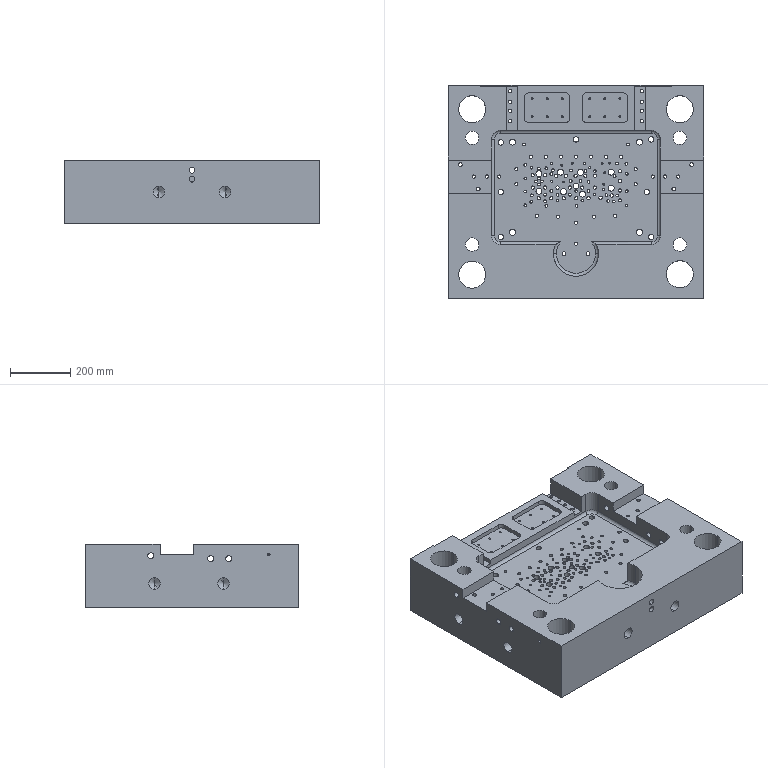Part | SolidWorks | features BaseBody 1 | 1 solid | 699 faces | box 850 x 710 x 210 mm | volume 93644180 mm3 | cylinder 499 | cone 106 | plane 87 | torus 7 | commonest cylinder face diameters 11 x110 9 x94 20 x57 6.8 x40 18 x32 26 x17